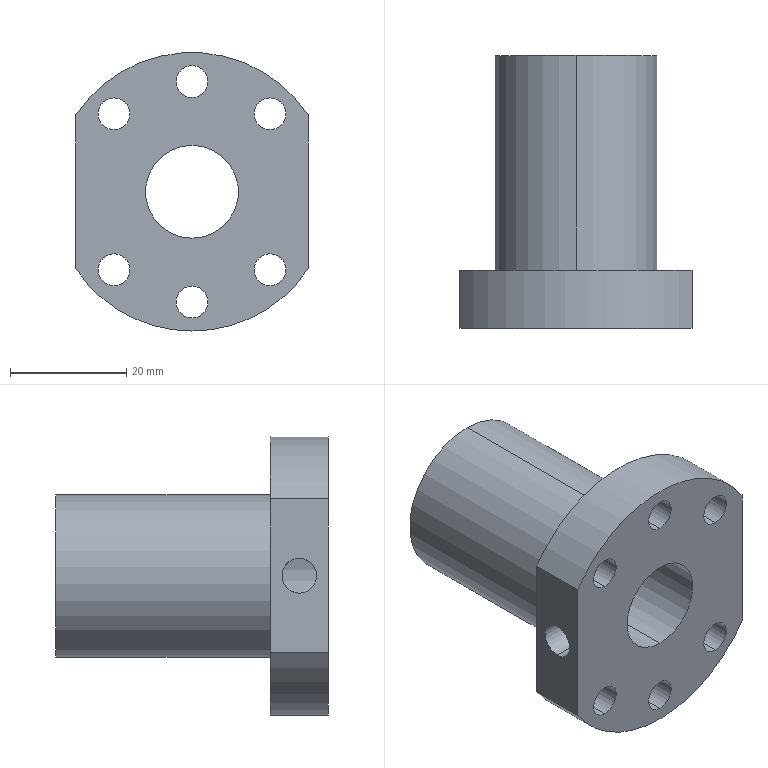Part | SolidWorks | features BaseBody 1 | 1 solid | 26 faces | box 40 x 47 x 48 mm | volume 28219 mm3 | cylinder 21 | plane 5 | commonest cylinder face diameters 5.5 x12 48 x3 6 x2 16 x2 28 x2
STEP:
#1=CARTESIAN_POINT('',(0.,47.,-14.));
#2=VERTEX_POINT('',#1);
#3=CARTESIAN_POINT('',(0.,47.,14.));
#4=VERTEX_POINT('',#3);
#5=CARTESIAN_POINT('',(0.,47.,0.));
#6=DIRECTION('',(0.,-1.,0.));
#7=DIRECTION('',(0.,0.,-1.));
#8=AXIS2_PLACEMENT_3D('',#5,#6,#7);
#9=CIRCLE('',#8,14.);
#10=EDGE_CURVE('',#2,#4,#9,.T.);
#11=ORIENTED_EDGE('',*,*,#10,.T.);
#12=CARTESIAN_POINT('',(0.,10.,14.));
#13=VERTEX_POINT('',#12);
#14=CARTESIAN_POINT('',(0.,47.,14.));
#15=DIRECTION('',(0.,-1.,0.));
#16=VECTOR('',#15,1000.);
#17=LINE('',#14,#16);
#18=EDGE_CURVE('',#4,#13,#17,.T.);
#19=ORIENTED_EDGE('',*,*,#18,.T.);
#20=CARTESIAN_POINT('',(0.,10.,-14.));
#21=VERTEX_POINT('',#20);
#22=CARTESIAN_POINT('',(0.,10.,0.));
#23=DIRECTION('',(0.,1.,0.));
#24=DIRECTION('',(0.,0.,-1.));
#25=AXIS2_PLACEMENT_3D('',#22,#23,#24);
#26=CIRCLE('',#25,14.);
#27=EDGE_CURVE('',#13,#21,#26,.T.);
#28=ORIENTED_EDGE('',*,*,#27,.T.);
#29=CARTESIAN_POINT('',(0.,47.,-14.));
#30=DIRECTION('',(0.,-1.,0.));
#31=VECTOR('',#30,1000.);
#32=LINE('',#29,#31);
#33=EDGE_CURVE('',#2,#21,#32,.T.);
#34=ORIENTED_EDGE('',*,*,#33,.F.);
#35=EDGE_LOOP('',(#11,#19,#28,#34));
#36=FACE_OUTER_BOUND('',#35,.T.);
#37=CARTESIAN_POINT('',(0.,47.,0.));
#38=DIRECTION('',(0.,-1.,0.));
#39=DIRECTION('',(0.,0.,-1.));
#40=AXIS2_PLACEMENT_3D('',#37,#38,#39);
#41=CYLINDRICAL_SURFACE('',#40,14.);
#42=ADVANCED_FACE('',(#36),#41,.T.);
#43=CARTESIAN_POINT('',(-13.435,10.,-10.685));
#44=VERTEX_POINT('',#43);
#45=CARTESIAN_POINT('',(-13.435,10.,-16.185));
#46=VERTEX_POINT('',#45);
#47=CARTESIAN_POINT('',(-13.435,10.,-13.435));
#48=DIRECTION('',(0.,-1.,0.));
#49=DIRECTION('',(0.,0.,-1.));
#50=AXIS2_PLACEMENT_3D('',#47,#48,#49);
#51=CIRCLE('',#50,2.75);
#52=EDGE_CURVE('',#44,#46,#51,.T.);
#53=ORIENTED_EDGE('',*,*,#52,.F.);
#54=CARTESIAN_POINT('',(-13.435,0.,-10.685));
#55=VERTEX_POINT('',#54);
#56=CARTESIAN_POINT('',(-13.435,10.,-10.685));
#57=DIRECTION('',(0.,-1.,0.));
#58=VECTOR('',#57,1000.);
#59=LINE('',#56,#58);
#60=EDGE_CURVE('',#44,#55,#59,.T.);
#61=ORIENTED_EDGE('',*,*,#60,.T.);
#62=CARTESIAN_POINT('',(-13.435,0.,-16.185));
#63=VERTEX_POINT('',#62);
#64=CARTESIAN_POINT('',(-13.435,0.,-13.435));
#65=DIRECTION('',(0.,1.,0.));
#66=DIRECTION('',(0.,0.,-1.));
#67=AXIS2_PLACEMENT_3D('',#64,#65,#66);
#68=CIRCLE('',#67,2.75);
#69=EDGE_CURVE('',#63,#55,#68,.T.);
#70=ORIENTED_EDGE('',*,*,#69,.F.);
#71=CARTESIAN_POINT('',(-13.435,10.,-16.185));
#72=DIRECTION('',(0.,-1.,0.));
#73=VECTOR('',#72,1000.);
#74=LINE('',#71,#73);
#75=EDGE_CURVE('',#46,#63,#74,.T.);
#76=ORIENTED_EDGE('',*,*,#75,.F.);
#77=EDGE_LOOP('',(#53,#61,#70,#76));
#78=FACE_OUTER_BOUND('',#77,.T.);
#79=CARTESIAN_POINT('',(-13.435,10.,-13.435));
#80=DIRECTION('',(0.,-1.,0.));
#81=DIRECTION('',(0.,0.,-1.));
#82=AXIS2_PLACEMENT_3D('',#79,#80,#81);
#83=CYLINDRICAL_SURFACE('',#82,2.75);
#84=ADVANCED_FACE('',(#78),#83,.F.);
#85=CARTESIAN_POINT('',(13.435,10.,16.185));
#86=VERTEX_POINT('',#85);
#87=CARTESIAN_POINT('',(13.435,10.,10.685));
#88=VERTEX_POINT('',#87);
#89=CARTESIAN_POINT('',(13.435,10.,13.435));
#90=DIRECTION('',(0.,-1.,0.));
#91=DIRECTION('',(0.,0.,-1.));
#92=AXIS2_PLACEMENT_3D('',#89,#90,#91);
#93=CIRCLE('',#92,2.75);
#94=EDGE_CURVE('',#86,#88,#93,.T.);
#95=ORIENTED_EDGE('',*,*,#94,.F.);
#96=CARTESIAN_POINT('',(13.435,0.,16.185));
#97=VERTEX_POINT('',#96);
#98=CARTESIAN_POINT('',(13.435,10.,16.185));
#99=DIRECTION('',(0.,-1.,0.));
#100=VECTOR('',#99,1000.);
#101=LINE('',#98,#100);
#102=EDGE_CURVE('',#86,#97,#101,.T.);
#103=ORIENTED_EDGE('',*,*,#102,.T.);
#104=CARTESIAN_POINT('',(13.435,0.,10.685));
#105=VERTEX_POINT('',#104);
#106=CARTESIAN_POINT('',(13.435,0.,13.435));
#107=DIRECTION('',(0.,1.,0.));
#108=DIRECTION('',(0.,0.,-1.));
#109=AXIS2_PLACEMENT_3D('',#106,#107,#108);
#110=CIRCLE('',#109,2.75);
#111=EDGE_CURVE('',#105,#97,#110,.T.);
#112=ORIENTED_EDGE('',*,*,#111,.F.);
#113=CARTESIAN_POINT('',(13.435,10.,10.685));
#114=DIRECTION('',(0.,-1.,0.));
#115=VECTOR('',#114,1000.);
#116=LINE('',#113,#115);
#117=EDGE_CURVE('',#88,#105,#116,.T.);
#118=ORIENTED_EDGE('',*,*,#117,.F.);
#119=EDGE_LOOP('',(#95,#103,#112,#118));
#120=FACE_OUTER_BOUND('',#119,.T.);
#121=CARTESIAN_POINT('',(13.435,10.,13.435));
#122=DIRECTION('',(0.,-1.,0.));
#123=DIRECTION('',(0.,0.,-1.));
#124=AXIS2_PLACEMENT_3D('',#121,#122,#123);
#125=CYLINDRICAL_SURFACE('',#124,2.75);
#126=ADVANCED_FACE('',(#120),#125,.F.);
#127=CARTESIAN_POINT('',(-13.435,10.,16.185));
#128=VERTEX_POINT('',#127);
#129=CARTESIAN_POINT('',(-13.435,10.,10.685));
#130=VERTEX_POINT('',#129);
#131=CARTESIAN_POINT('',(-13.435,10.,13.435));
#132=DIRECTION('',(0.,-1.,0.));
#133=DIRECTION('',(0.,0.,-1.));
#134=AXIS2_PLACEMENT_3D('',#131,#132,#133);
#135=CIRCLE('',#134,2.75);
#136=EDGE_CURVE('',#128,#130,#135,.T.);
#137=ORIENTED_EDGE('',*,*,#136,.F.);
#138=CARTESIAN_POINT('',(-13.435,0.,16.185));
#139=VERTEX_POINT('',#138);
#140=CARTESIAN_POINT('',(-13.435,10.,16.185));
#141=DIRECTION('',(0.,-1.,0.));
#142=VECTOR('',#141,1000.);
#143=LINE('',#140,#142);
#144=EDGE_CURVE('',#128,#139,#143,.T.);
#145=ORIENTED_EDGE('',*,*,#144,.T.);
#146=CARTESIAN_POINT('',(-13.435,0.,10.685));
#147=VERTEX_POINT('',#146);
#148=CARTESIAN_POINT('',(-13.435,0.,13.435));
#149=DIRECTION('',(0.,1.,0.));
#150=DIRECTION('',(0.,0.,-1.));
#151=AXIS2_PLACEMENT_3D('',#148,#149,#150);
#152=CIRCLE('',#151,2.75);
#153=EDGE_CURVE('',#147,#139,#152,.T.);
#154=ORIENTED_EDGE('',*,*,#153,.F.);
#155=CARTESIAN_POINT('',(-13.435,10.,10.685));
#156=DIRECTION('',(0.,-1.,0.));
#157=VECTOR('',#156,1000.);
#158=LINE('',#155,#157);
#159=EDGE_CURVE('',#130,#147,#158,.T.);
#160=ORIENTED_EDGE('',*,*,#159,.F.);
#161=EDGE_LOOP('',(#137,#145,#154,#160));
#162=FACE_OUTER_BOUND('',#161,.T.);
#163=CARTESIAN_POINT('',(-13.435,10.,13.435));
#164=DIRECTION('',(0.,-1.,0.));
#165=DIRECTION('',(0.,0.,-1.));
#166=AXIS2_PLACEMENT_3D('',#163,#164,#165);
#167=CYLINDRICAL_SURFACE('',#166,2.75);
#168=ADVANCED_FACE('',(#162),#167,.F.);
#169=CARTESIAN_POINT('',(0.,10.,21.75));
#170=VERTEX_POINT('',#169);
#171=CARTESIAN_POINT('',(0.,10.,16.25));
#172=VERTEX_POINT('',#171);
#173=CARTESIAN_POINT('',(0.,10.,19.));
#174=DIRECTION('',(0.,-1.,0.));
#175=DIRECTION('',(0.,0.,-1.));
#176=AXIS2_PLACEMENT_3D('',#173,#174,#175);
#177=CIRCLE('',#176,2.75);
#178=EDGE_CURVE('',#170,#172,#177,.T.);
#179=ORIENTED_EDGE('',*,*,#178,.F.);
#180=CARTESIAN_POINT('',(0.,0.,21.75));
#181=VERTEX_POINT('',#180);
#182=CARTESIAN_POINT('',(0.,10.,21.75));
#183=DIRECTION('',(0.,-1.,0.));
#184=VECTOR('',#183,1000.);
#185=LINE('',#182,#184);
#186=EDGE_CURVE('',#170,#181,#185,.T.);
#187=ORIENTED_EDGE('',*,*,#186,.T.);
#188=CARTESIAN_POINT('',(0.,0.,16.25));
#189=VERTEX_POINT('',#188);
#190=CARTESIAN_POINT('',(0.,0.,19.));
#191=DIRECTION('',(0.,1.,0.));
#192=DIRECTION('',(0.,0.,-1.));
#193=AXIS2_PLACEMENT_3D('',#190,#191,#192);
#194=CIRCLE('',#193,2.75);
#195=EDGE_CURVE('',#189,#181,#194,.T.);
#196=ORIENTED_EDGE('',*,*,#195,.F.);
#197=CARTESIAN_POINT('',(0.,10.,16.25));
#198=DIRECTION('',(0.,-1.,0.));
#199=VECTOR('',#198,1000.);
#200=LINE('',#197,#199);
#201=EDGE_CURVE('',#172,#189,#200,.T.);
#202=ORIENTED_EDGE('',*,*,#201,.F.);
#203=EDGE_LOOP('',(#179,#187,#196,#202));
#204=FACE_OUTER_BOUND('',#203,.T.);
#205=CARTESIAN_POINT('',(0.,10.,19.));
#206=DIRECTION('',(0.,-1.,0.));
#207=DIRECTION('',(0.,0.,-1.));
#208=AXIS2_PLACEMENT_3D('',#205,#206,#207);
#209=CYLINDRICAL_SURFACE('',#208,2.75);
#210=ADVANCED_FACE('',(#204),#209,.F.);
#211=CARTESIAN_POINT('',(0.,10.,-24.));
#212=VERTEX_POINT('',#211);
#213=CARTESIAN_POINT('',(-20.,10.,-13.266));
#214=VERTEX_POINT('',#213);
#215=CARTESIAN_POINT('',(0.,10.,0.));
#216=DIRECTION('',(0.,1.,0.));
#217=DIRECTION('',(0.,0.,-1.));
#218=AXIS2_PLACEMENT_3D('',#215,#216,#217);
#219=CIRCLE('',#218,24.);
#220=EDGE_CURVE('',#212,#214,#219,.T.);
#221=ORIENTED_EDGE('',*,*,#220,.F.);
#222=CARTESIAN_POINT('',(0.,0.,-24.));
#223=VERTEX_POINT('',#222);
#224=CARTESIAN_POINT('',(0.,10.,-24.));
#225=DIRECTION('',(0.,-1.,0.));
#226=VECTOR('',#225,1000.);
#227=LINE('',#224,#226);
#228=EDGE_CURVE('',#212,#223,#227,.T.);
#229=ORIENTED_EDGE('',*,*,#228,.T.);
#230=CARTESIAN_POINT('',(-20.,0.,-13.266));
#231=VERTEX_POINT('',#230);
#232=CARTESIAN_POINT('',(0.,0.,0.));
#233=DIRECTION('',(0.,1.,0.));
#234=DIRECTION('',(0.,0.,-1.));
#235=AXIS2_PLACEMENT_3D('',#232,#233,#234);
#236=CIRCLE('',#235,24.);
#237=EDGE_CURVE('',#223,#231,#236,.T.);
#238=ORIENTED_EDGE('',*,*,#237,.T.);
#239=CARTESIAN_POINT('',(-20.,10.,-13.266));
#240=DIRECTION('',(0.,1.,0.));
#241=VECTOR('',#240,1000.);
#242=LINE('',#239,#241);
#243=EDGE_CURVE('',#231,#214,#242,.T.);
#244=ORIENTED_EDGE('',*,*,#243,.T.);
#245=EDGE_LOOP('',(#221,#229,#238,#244));
#246=FACE_OUTER_BOUND('',#245,.T.);
#247=CARTESIAN_POINT('',(0.,10.,0.));
#248=DIRECTION('',(0.,-1.,0.));
#249=DIRECTION('',(0.,0.,-1.));
#250=AXIS2_PLACEMENT_3D('',#247,#248,#249);
#251=CYLINDRICAL_SURFACE('',#250,24.);
#252=ADVANCED_FACE('',(#246),#251,.T.);
#253=CARTESIAN_POINT('',(13.435,10.,-10.685));
#254=VERTEX_POINT('',#253);
#255=CARTESIAN_POINT('',(13.435,10.,-16.185));
#256=VERTEX_POINT('',#255);
#257=CARTESIAN_POINT('',(13.435,10.,-13.435));
#258=DIRECTION('',(0.,-1.,0.));
#259=DIRECTION('',(0.,0.,-1.));
#260=AXIS2_PLACEMENT_3D('',#257,#258,#259);
#261=CIRCLE('',#260,2.75);
#262=EDGE_CURVE('',#254,#256,#261,.T.);
#263=ORIENTED_EDGE('',*,*,#262,.F.);
#264=CARTESIAN_POINT('',(13.435,0.,-10.685));
#265=VERTEX_POINT('',#264);
#266=CARTESIAN_POINT('',(13.435,10.,-10.685));
#267=DIRECTION('',(0.,-1.,0.));
#268=VECTOR('',#267,1000.);
#269=LINE('',#266,#268);
#270=EDGE_CURVE('',#254,#265,#269,.T.);
#271=ORIENTED_EDGE('',*,*,#270,.T.);
#272=CARTESIAN_POINT('',(13.435,0.,-16.185));
#273=VERTEX_POINT('',#272);
#274=CARTESIAN_POINT('',(13.435,0.,-13.435));
#275=DIRECTION('',(0.,1.,0.));
#276=DIRECTION('',(0.,0.,-1.));
#277=AXIS2_PLACEMENT_3D('',#274,#275,#276);
#278=CIRCLE('',#277,2.75);
#279=EDGE_CURVE('',#273,#265,#278,.T.);
#280=ORIENTED_EDGE('',*,*,#279,.F.);
#281=CARTESIAN_POINT('',(13.435,10.,-16.185));
#282=DIRECTION('',(0.,-1.,0.));
#283=VECTOR('',#282,1000.);
#284=LINE('',#281,#283);
#285=EDGE_CURVE('',#256,#273,#284,.T.);
#286=ORIENTED_EDGE('',*,*,#285,.F.);
#287=EDGE_LOOP('',(#263,#271,#280,#286));
#288=FACE_OUTER_BOUND('',#287,.T.);
#289=CARTESIAN_POINT('',(13.435,10.,-13.435));
#290=DIRECTION('',(0.,-1.,0.));
#291=DIRECTION('',(0.,0.,-1.));
#292=AXIS2_PLACEMENT_3D('',#289,#290,#291);
#293=CYLINDRICAL_SURFACE('',#292,2.75);
#294=ADVANCED_FACE('',(#288),#293,.F.);
#295=CARTESIAN_POINT('',(0.,10.,-16.25));
#296=VERTEX_POINT('',#295);
#297=CARTESIAN_POINT('',(0.,10.,-21.75));
#298=VERTEX_POINT('',#297);
#299=CARTESIAN_POINT('',(0.,10.,-19.));
#300=DIRECTION('',(0.,-1.,0.));
#301=DIRECTION('',(0.,0.,-1.));
#302=AXIS2_PLACEMENT_3D('',#299,#300,#301);
#303=CIRCLE('',#302,2.75);
#304=EDGE_CURVE('',#296,#298,#303,.T.);
#305=ORIENTED_EDGE('',*,*,#304,.F.);
#306=CARTESIAN_POINT('',(0.,0.,-16.25));
#307=VERTEX_POINT('',#306);
#308=CARTESIAN_POINT('',(0.,10.,-16.25));
#309=DIRECTION('',(0.,-1.,0.));
#310=VECTOR('',#309,1000.);
#311=LINE('',#308,#310);
#312=EDGE_CURVE('',#296,#307,#311,.T.);
#313=ORIENTED_EDGE('',*,*,#312,.T.);
#314=CARTESIAN_POINT('',(0.,0.,-21.75));
#315=VERTEX_POINT('',#314);
#316=CARTESIAN_POINT('',(0.,0.,-19.));
#317=DIRECTION('',(0.,1.,0.));
#318=DIRECTION('',(0.,0.,-1.));
#319=AXIS2_PLACEMENT_3D('',#316,#317,#318);
#320=CIRCLE('',#319,2.75);
#321=EDGE_CURVE('',#315,#307,#320,.T.);
#322=ORIENTED_EDGE('',*,*,#321,.F.);
#323=CARTESIAN_POINT('',(0.,10.,-21.75));
#324=DIRECTION('',(0.,-1.,0.));
#325=VECTOR('',#324,1000.);
#326=LINE('',#323,#325);
#327=EDGE_CURVE('',#298,#315,#326,.T.);
#328=ORIENTED_EDGE('',*,*,#327,.F.);
#329=EDGE_LOOP('',(#305,#313,#322,#328));
#330=FACE_OUTER_BOUND('',#329,.T.);
#331=CARTESIAN_POINT('',(0.,10.,-19.));
#332=DIRECTION('',(0.,-1.,0.));
#333=DIRECTION('',(0.,0.,-1.));
#334=AXIS2_PLACEMENT_3D('',#331,#332,#333);
#335=CYLINDRICAL_SURFACE('',#334,2.75);
#336=ADVANCED_FACE('',(#330),#335,.F.);
#337=CARTESIAN_POINT('',(-7.416,5.,3.));
#338=VERTEX_POINT('',#337);
#339=CARTESIAN_POINT('',(-7.416,5.,-3.));
#340=VERTEX_POINT('',#339);
#341=CARTESIAN_POINT('',(-7.416,5.,3.));
#342=CARTESIAN_POINT('',(-7.416,4.8,3.));
#343=CARTESIAN_POINT('',(-7.424,4.603,2.98));
#344=CARTESIAN_POINT('',(-7.455,4.218,2.903));
#345=CARTESIAN_POINT('',(-7.478,4.026,2.844));
#346=CARTESIAN_POINT('',(-7.533,3.664,2.693));
#347=CARTESIAN_POINT('',(-7.566,3.493,2.601));
#348=CARTESIAN_POINT('',(-7.637,3.168,2.384));
#349=CARTESIAN_POINT('',(-7.676,3.016,2.259));
#350=CARTESIAN_POINT('',(-7.789,2.605,1.848));
#351=CARTESIAN_POINT('',(-7.863,2.382,1.516));
#352=CARTESIAN_POINT('',(-7.942,2.157,0.9761));
#353=CARTESIAN_POINT('',(-7.964,2.098,0.7852));
#354=CARTESIAN_POINT('',(-7.993,2.02,0.3971));
#355=CARTESIAN_POINT('',(-8.,2.,0.2012));
#356=CARTESIAN_POINT('',(-8.,2.,-0.1942));
#357=CARTESIAN_POINT('',(-7.993,2.02,-0.3949));
#358=CARTESIAN_POINT('',(-7.964,2.097,-0.7814));
#359=CARTESIAN_POINT('',(-7.943,2.154,-0.9694));
#360=CARTESIAN_POINT('',(-7.89,2.306,-1.335));
#361=CARTESIAN_POINT('',(-7.858,2.399,-1.507));
#362=CARTESIAN_POINT('',(-7.789,2.615,-1.831));
#363=CARTESIAN_POINT('',(-7.752,2.741,-1.983));
#364=CARTESIAN_POINT('',(-7.676,3.016,-2.259));
#365=CARTESIAN_POINT('',(-7.638,3.165,-2.382));
#366=CARTESIAN_POINT('',(-7.567,3.489,-2.599));
#367=CARTESIAN_POINT('',(-7.534,3.664,-2.693));
#368=CARTESIAN_POINT('',(-7.478,4.024,-2.844));
#369=CARTESIAN_POINT('',(-7.456,4.211,-2.901));
#370=CARTESIAN_POINT('',(-7.424,4.6,-2.98));
#371=CARTESIAN_POINT('',(-7.416,4.8,-3.));
#372=CARTESIAN_POINT('',(-7.416,5.,-3.));
#373=B_SPLINE_CURVE_WITH_KNOTS('',3,(#341,#342,#343,#344,#345,#346,#347,#348,#349,#350,#351,#352,#353,#354,#355,#356,#357,#358,#359,#360,#361,#362,#363,#364,#365,#366,#367,#368,#369,#370,#371,#372),.UNSPECIFIED.,.F.,.F.,(4,2,2,2,2,2,2,2,2,2,2,2,2,2,2,4),(0.,0.0005914,0.001183,0.001774,0.002366,0.003548,0.00414,0.004731,0.005323,0.005914,0.006505,0.007097,0.007688,0.00828,0.008871,0.009462),.UNSPECIFIED.);
#374=EDGE_CURVE('',#338,#340,#373,.T.);
#375=ORIENTED_EDGE('',*,*,#374,.F.);
#376=CARTESIAN_POINT('',(-7.416,5.,-3.));
#377=CARTESIAN_POINT('',(-7.416,5.2,-3.));
#378=CARTESIAN_POINT('',(-7.424,5.397,-2.98));
#379=CARTESIAN_POINT('',(-7.455,5.782,-2.903));
#380=CARTESIAN_POINT('',(-7.478,5.974,-2.844));
#381=CARTESIAN_POINT('',(-7.533,6.336,-2.693));
#382=CARTESIAN_POINT('',(-7.566,6.507,-2.601));
#383=CARTESIAN_POINT('',(-7.637,6.832,-2.384));
#384=CARTESIAN_POINT('',(-7.676,6.984,-2.259));
#385=CARTESIAN_POINT('',(-7.789,7.395,-1.848));
#386=CARTESIAN_POINT('',(-7.863,7.618,-1.516));
#387=CARTESIAN_POINT('',(-7.942,7.843,-0.9761));
#388=CARTESIAN_POINT('',(-7.964,7.902,-0.7852));
#389=CARTESIAN_POINT('',(-7.993,7.98,-0.3971));
#390=CARTESIAN_POINT('',(-8.,8.,-0.2012));
#391=CARTESIAN_POINT('',(-8.,8.,0.1942));
#392=CARTESIAN_POINT('',(-7.993,7.98,0.3949));
#393=CARTESIAN_POINT('',(-7.964,7.903,0.7814));
#394=CARTESIAN_POINT('',(-7.943,7.846,0.9694));
#395=CARTESIAN_POINT('',(-7.89,7.694,1.335));
#396=CARTESIAN_POINT('',(-7.858,7.601,1.507));
#397=CARTESIAN_POINT('',(-7.789,7.385,1.831));
#398=CARTESIAN_POINT('',(-7.752,7.259,1.983));
#399=CARTESIAN_POINT('',(-7.676,6.984,2.259));
#400=CARTESIAN_POINT('',(-7.638,6.835,2.382));
#401=CARTESIAN_POINT('',(-7.567,6.511,2.599));
#402=CARTESIAN_POINT('',(-7.534,6.336,2.693));
#403=CARTESIAN_POINT('',(-7.478,5.976,2.844));
#404=CARTESIAN_POINT('',(-7.456,5.789,2.901));
#405=CARTESIAN_POINT('',(-7.424,5.4,2.98));
#406=CARTESIAN_POINT('',(-7.416,5.2,3.));
#407=CARTESIAN_POINT('',(-7.416,5.,3.));
#408=B_SPLINE_CURVE_WITH_KNOTS('',3,(#376,#377,#378,#379,#380,#381,#382,#383,#384,#385,#386,#387,#388,#389,#390,#391,#392,#393,#394,#395,#396,#397,#398,#399,#400,#401,#402,#403,#404,#405,#406,#407),.UNSPECIFIED.,.F.,.F.,(4,2,2,2,2,2,2,2,2,2,2,2,2,2,2,4),(0.009462,0.01005,0.01064,0.01124,0.01183,0.01301,0.0136,0.01419,0.01478,0.01538,0.01597,0.01656,0.01715,0.01774,0.01833,0.01892),.UNSPECIFIED.);
#409=EDGE_CURVE('',#340,#338,#408,.T.);
#410=ORIENTED_EDGE('',*,*,#409,.F.);
#411=EDGE_LOOP('',(#375,#410));
#412=FACE_BOUND('',#411,.T.);
#413=CARTESIAN_POINT('',(0.,47.,8.));
#414=VERTEX_POINT('',#413);
#415=CARTESIAN_POINT('',(0.,47.,-8.));
#416=VERTEX_POINT('',#415);
#417=CARTESIAN_POINT('',(0.,47.,0.));
#418=DIRECTION('',(0.,-1.,0.));
#419=DIRECTION('',(0.,0.,-1.));
#420=AXIS2_PLACEMENT_3D('',#417,#418,#419);
#421=CIRCLE('',#420,8.);
#422=EDGE_CURVE('',#414,#416,#421,.T.);
#423=ORIENTED_EDGE('',*,*,#422,.F.);
#424=CARTESIAN_POINT('',(0.,0.,8.));
#425=VERTEX_POINT('',#424);
#426=CARTESIAN_POINT('',(0.,47.,8.));
#427=DIRECTION('',(0.,-1.,0.));
#428=VECTOR('',#427,1000.);
#429=LINE('',#426,#428);
#430=EDGE_CURVE('',#414,#425,#429,.T.);
#431=ORIENTED_EDGE('',*,*,#430,.T.);
#432=CARTESIAN_POINT('',(0.,0.,-8.));
#433=VERTEX_POINT('',#432);
#434=CARTESIAN_POINT('',(0.,0.,0.));
#435=DIRECTION('',(0.,1.,0.));
#436=DIRECTION('',(0.,0.,-1.));
#437=AXIS2_PLACEMENT_3D('',#434,#435,#436);
#438=CIRCLE('',#437,8.);
#439=EDGE_CURVE('',#433,#425,#438,.T.);
#440=ORIENTED_EDGE('',*,*,#439,.F.);
#441=CARTESIAN_POINT('',(0.,47.,-8.));
#442=DIRECTION('',(0.,-1.,0.));
#443=VECTOR('',#442,1000.);
#444=LINE('',#441,#443);
#445=EDGE_CURVE('',#416,#433,#444,.T.);
#446=ORIENTED_EDGE('',*,*,#445,.F.);
#447=EDGE_LOOP('',(#423,#431,#440,#446));
#448=FACE_OUTER_BOUND('',#447,.T.);
#449=CARTESIAN_POINT('',(0.,47.,0.));
#450=DIRECTION('',(0.,-1.,0.));
#451=DIRECTION('',(0.,0.,-1.));
#452=AXIS2_PLACEMENT_3D('',#449,#450,#451);
#453=CYLINDRICAL_SURFACE('',#452,8.);
#454=ADVANCED_FACE('',(#412,#448),#453,.F.);
#455=ORIENTED_EDGE('',*,*,#374,.T.);
#456=CARTESIAN_POINT('',(-20.,5.,-3.));
#457=VERTEX_POINT('',#456);
#458=CARTESIAN_POINT('',(0.,5.,-3.));
#459=DIRECTION('',(-1.,0.,0.));
#460=VECTOR('',#459,1000.);
#461=LINE('',#458,#460);
#462=EDGE_CURVE('',#340,#457,#461,.T.);
#463=ORIENTED_EDGE('',*,*,#462,.T.);
#464=CARTESIAN_POINT('',(-20.,5.,3.));
#465=VERTEX_POINT('',#464);
#466=CARTESIAN_POINT('',(-20.,5.,0.));
#467=DIRECTION('',(-1.,0.,0.));
#468=DIRECTION('',(0.,0.,1.));
#469=AXIS2_PLACEMENT_3D('',#466,#467,#468);
#470=CIRCLE('',#469,3.);
#471=EDGE_CURVE('',#457,#465,#470,.T.);
#472=ORIENTED_EDGE('',*,*,#471,.T.);
#473=CARTESIAN_POINT('',(0.,5.,3.));
#474=DIRECTION('',(-1.,0.,0.));
#475=VECTOR('',#474,1000.);
#476=LINE('',#473,#475);
#477=EDGE_CURVE('',#338,#465,#476,.T.);
#478=ORIENTED_EDGE('',*,*,#477,.F.);
#479=EDGE_LOOP('',(#455,#463,#472,#478));
#480=FACE_OUTER_BOUND('',#479,.T.);
#481=CARTESIAN_POINT('',(0.,5.,0.));
#482=DIRECTION('',(-1.,0.,0.));
#483=DIRECTION('',(0.,0.,1.));
#484=AXIS2_PLACEMENT_3D('',#481,#482,#483);
#485=CYLINDRICAL_SURFACE('',#484,3.);
#486=ADVANCED_FACE('',(#480),#485,.F.);
#487=ORIENTED_EDGE('',*,*,#18,.F.);
#488=CARTESIAN_POINT('',(0.,47.,0.));
#489=DIRECTION('',(0.,-1.,0.));
#490=DIRECTION('',(0.,0.,-1.));
#491=AXIS2_PLACEMENT_3D('',#488,#489,#490);
#492=CIRCLE('',#491,14.);
#493=EDGE_CURVE('',#4,#2,#492,.T.);
#494=ORIENTED_EDGE('',*,*,#493,.T.);
#495=ORIENTED_EDGE('',*,*,#33,.T.);
#496=CARTESIAN_POINT('',(0.,10.,0.));
#497=DIRECTION('',(0.,1.,0.));
#498=DIRECTION('',(0.,0.,-1.));
#499=AXIS2_PLACEMENT_3D('',#496,#497,#498);
#500=CIRCLE('',#499,14.);
#501=EDGE_CURVE('',#21,#13,#500,.T.);
#502=ORIENTED_EDGE('',*,*,#501,.T.);
#503=EDGE_LOOP('',(#487,#494,#495,#502));
#504=FACE_OUTER_BOUND('',#503,.T.);
#505=CARTESIAN_POINT('',(0.,47.,0.));
#506=DIRECTION('',(0.,-1.,0.));
#507=DIRECTION('',(0.,0.,-1.));
#508=AXIS2_PLACEMENT_3D('',#505,#506,#507);
#509=CYLINDRICAL_SURFACE('',#508,14.);
#510=ADVANCED_FACE('',(#504),#509,.T.);
#511=CARTESIAN_POINT('',(-13.435,10.,-13.435));
#512=DIRECTION('',(0.,-1.,0.));
#513=DIRECTION('',(0.,0.,-1.));
#514=AXIS2_PLACEMENT_3D('',#511,#512,#513);
#515=CIRCLE('',#514,2.75);
#516=EDGE_CURVE('',#46,#44,#515,.T.);
#517=ORIENTED_EDGE('',*,*,#516,.T.);
#518=ORIENTED_EDGE('',*,*,#52,.T.);
#519=EDGE_LOOP('',(#517,#518));
#520=FACE_BOUND('',#519,.T.);
#521=CARTESIAN_POINT('',(13.435,10.,13.435));
#522=DIRECTION('',(0.,-1.,0.));
#523=DIRECTION('',(0.,0.,-1.));
#524=AXIS2_PLACEMENT_3D('',#521,#522,#523);
#525=CIRCLE('',#524,2.75);
#526=EDGE_CURVE('',#88,#86,#525,.T.);
#527=ORIENTED_EDGE('',*,*,#526,.T.);
#528=ORIENTED_EDGE('',*,*,#94,.T.);
#529=EDGE_LOOP('',(#527,#528));
#530=FACE_BOUND('',#529,.T.);
#531=CARTESIAN_POINT('',(-13.435,10.,13.435));
#532=DIRECTION('',(0.,-1.,0.));
#533=DIRECTION('',(0.,0.,-1.));
#534=AXIS2_PLACEMENT_3D('',#531,#532,#533);
#535=CIRCLE('',#534,2.75);
#536=EDGE_CURVE('',#130,#128,#535,.T.);
#537=ORIENTED_EDGE('',*,*,#536,.T.);
#538=ORIENTED_EDGE('',*,*,#136,.T.);
#539=EDGE_LOOP('',(#537,#538));
#540=FACE_BOUND('',#539,.T.);
#541=CARTESIAN_POINT('',(0.,10.,19.));
#542=DIRECTION('',(0.,-1.,0.));
#543=DIRECTION('',(0.,0.,-1.));
#544=AXIS2_PLACEMENT_3D('',#541,#542,#543);
#545=CIRCLE('',#544,2.75);
#546=EDGE_CURVE('',#172,#170,#545,.T.);
#547=ORIENTED_EDGE('',*,*,#546,.T.);
#548=ORIENTED_EDGE('',*,*,#178,.T.);
#549=EDGE_LOOP('',(#547,#548));
#550=FACE_BOUND('',#549,.T.);
#551=ORIENTED_EDGE('',*,*,#501,.F.);
#552=ORIENTED_EDGE('',*,*,#27,.F.);
#553=EDGE_LOOP('',(#551,#552));
#554=FACE_BOUND('',#553,.T.);
#555=CARTESIAN_POINT('',(-20.,10.,13.266));
#556=VERTEX_POINT('',#555);
#557=CARTESIAN_POINT('',(-20.,10.,0.));
#558=DIRECTION('',(0.,0.,1.));
#559=VECTOR('',#558,1000.);
#560=LINE('',#557,#559);
#561=EDGE_CURVE('',#214,#556,#560,.T.);
#562=ORIENTED_EDGE('',*,*,#561,.T.);
#563=CARTESIAN_POINT('',(20.,10.,13.266));
#564=VERTEX_POINT('',#563);
#565=CARTESIAN_POINT('',(0.,10.,0.));
#566=DIRECTION('',(0.,1.,0.));
#567=DIRECTION('',(0.,0.,-1.));
#568=AXIS2_PLACEMENT_3D('',#565,#566,#567);
#569=CIRCLE('',#568,24.);
#570=EDGE_CURVE('',#556,#564,#569,.T.);
#571=ORIENTED_EDGE('',*,*,#570,.T.);
#572=CARTESIAN_POINT('',(20.,10.,-13.266));
#573=VERTEX_POINT('',#572);
#574=CARTESIAN_POINT('',(20.,10.,0.));
#575=DIRECTION('',(0.,0.,-1.));
#576=VECTOR('',#575,1000.);
#577=LINE('',#574,#576);
#578=EDGE_CURVE('',#564,#573,#577,.T.);
#579=ORIENTED_EDGE('',*,*,#578,.T.);
#580=CARTESIAN_POINT('',(0.,10.,0.));
#581=DIRECTION('',(0.,1.,0.));
#582=DIRECTION('',(0.,0.,-1.));
#583=AXIS2_PLACEMENT_3D('',#580,#581,#582);
#584=CIRCLE('',#583,24.);
#585=EDGE_CURVE('',#573,#212,#584,.T.);
#586=ORIENTED_EDGE('',*,*,#585,.T.);
#587=ORIENTED_EDGE('',*,*,#220,.T.);
#588=EDGE_LOOP('',(#562,#571,#579,#586,#587));
#589=FACE_OUTER_BOUND('',#588,.T.);
#590=CARTESIAN_POINT('',(13.435,10.,-13.435));
#591=DIRECTION('',(0.,-1.,0.));
#592=DIRECTION('',(0.,0.,-1.));
#593=AXIS2_PLACEMENT_3D('',#590,#591,#592);
#594=CIRCLE('',#593,2.75);
#595=EDGE_CURVE('',#256,#254,#594,.T.);
#596=ORIENTED_EDGE('',*,*,#595,.T.);
#597=ORIENTED_EDGE('',*,*,#262,.T.);
#598=EDGE_LOOP('',(#596,#597));
#599=FACE_BOUND('',#598,.T.);
#600=CARTESIAN_POINT('',(0.,10.,-19.));
#601=DIRECTION('',(0.,-1.,0.));
#602=DIRECTION('',(0.,0.,-1.));
#603=AXIS2_PLACEMENT_3D('',#600,#601,#602);
#604=CIRCLE('',#603,2.75);
#605=EDGE_CURVE('',#298,#296,#604,.T.);
#606=ORIENTED_EDGE('',*,*,#605,.T.);
#607=ORIENTED_EDGE('',*,*,#304,.T.);
#608=EDGE_LOOP('',(#606,#607));
#609=FACE_BOUND('',#608,.T.);
#610=CARTESIAN_POINT('',(0.,10.,0.));
#611=DIRECTION('',(0.,1.,0.));
#612=DIRECTION('',(0.,0.,1.));
#613=AXIS2_PLACEMENT_3D('',#610,#611,#612);
#614=PLANE('',#613);
#615=ADVANCED_FACE('',(#520,#530,#540,#550,#554,#589,#599,#609),#614,.T.);
#616=ORIENTED_EDGE('',*,*,#10,.F.);
#617=ORIENTED_EDGE('',*,*,#493,.F.);
#618=EDGE_LOOP('',(#616,#617));
#619=FACE_OUTER_BOUND('',#618,.T.);
#620=CARTESIAN_POINT('',(0.,47.,0.));
#621=DIRECTION('',(0.,-1.,0.));
#622=DIRECTION('',(0.,0.,-1.));
#623=AXIS2_PLACEMENT_3D('',#620,#621,#622);
#624=CIRCLE('',#623,8.);
#625=EDGE_CURVE('',#416,#414,#624,.T.);
#626=ORIENTED_EDGE('',*,*,#625,.T.);
#627=ORIENTED_EDGE('',*,*,#422,.T.);
#628=EDGE_LOOP('',(#626,#627));
#629=FACE_BOUND('',#628,.T.);
#630=CARTESIAN_POINT('',(0.,47.,0.));
#631=DIRECTION('',(0.,1.,0.));
#632=DIRECTION('',(0.,0.,1.));
#633=AXIS2_PLACEMENT_3D('',#630,#631,#632);
#634=PLANE('',#633);
#635=ADVANCED_FACE('',(#619,#629),#634,.T.);
#636=ORIENTED_EDGE('',*,*,#60,.F.);
#637=ORIENTED_EDGE('',*,*,#516,.F.);
#638=ORIENTED_EDGE('',*,*,#75,.T.);
#639=CARTESIAN_POINT('',(-13.435,0.,-13.435));
#640=DIRECTION('',(0.,1.,0.));
#641=DIRECTION('',(0.,0.,-1.));
#642=AXIS2_PLACEMENT_3D('',#639,#640,#641);
#643=CIRCLE('',#642,2.75);
#644=EDGE_CURVE('',#55,#63,#643,.T.);
#645=ORIENTED_EDGE('',*,*,#644,.F.);
#646=EDGE_LOOP('',(#636,#637,#638,#645));
#647=FACE_OUTER_BOUND('',#646,.T.);
#648=CARTESIAN_POINT('',(-13.435,10.,-13.435));
#649=DIRECTION('',(0.,-1.,0.));
#650=DIRECTION('',(0.,0.,-1.));
#651=AXIS2_PLACEMENT_3D('',#648,#649,#650);
#652=CYLINDRICAL_SURFACE('',#651,2.75);
#653=ADVANCED_FACE('',(#647),#652,.F.);
#654=ORIENTED_EDGE('',*,*,#102,.F.);
#655=ORIENTED_EDGE('',*,*,#526,.F.);
#656=ORIENTED_EDGE('',*,*,#117,.T.);
#657=CARTESIAN_POINT('',(13.435,0.,13.435));
#658=DIRECTION('',(0.,1.,0.));
#659=DIRECTION('',(0.,0.,-1.));
#660=AXIS2_PLACEMENT_3D('',#657,#658,#659);
#661=CIRCLE('',#660,2.75);
#662=EDGE_CURVE('',#97,#105,#661,.T.);
#663=ORIENTED_EDGE('',*,*,#662,.F.);
#664=EDGE_LOOP('',(#654,#655,#656,#663));
#665=FACE_OUTER_BOUND('',#664,.T.);
#666=CARTESIAN_POINT('',(13.435,10.,13.435));
#667=DIRECTION('',(0.,-1.,0.));
#668=DIRECTION('',(0.,0.,-1.));
#669=AXIS2_PLACEMENT_3D('',#666,#667,#668);
#670=CYLINDRICAL_SURFACE('',#669,2.75);
#671=ADVANCED_FACE('',(#665),#670,.F.);
#672=ORIENTED_EDGE('',*,*,#144,.F.);
#673=ORIENTED_EDGE('',*,*,#536,.F.);
#674=ORIENTED_EDGE('',*,*,#159,.T.);
#675=CARTESIAN_POINT('',(-13.435,0.,13.435));
#676=DIRECTION('',(0.,1.,0.));
#677=DIRECTION('',(0.,0.,-1.));
#678=AXIS2_PLACEMENT_3D('',#675,#676,#677);
#679=CIRCLE('',#678,2.75);
#680=EDGE_CURVE('',#139,#147,#679,.T.);
#681=ORIENTED_EDGE('',*,*,#680,.F.);
#682=EDGE_LOOP('',(#672,#673,#674,#681));
#683=FACE_OUTER_BOUND('',#682,.T.);
#684=CARTESIAN_POINT('',(-13.435,10.,13.435));
#685=DIRECTION('',(0.,-1.,0.));
#686=DIRECTION('',(0.,0.,-1.));
#687=AXIS2_PLACEMENT_3D('',#684,#685,#686);
#688=CYLINDRICAL_SURFACE('',#687,2.75);
#689=ADVANCED_FACE('',(#683),#688,.F.);
#690=ORIENTED_EDGE('',*,*,#186,.F.);
#691=ORIENTED_EDGE('',*,*,#546,.F.);
#692=ORIENTED_EDGE('',*,*,#201,.T.);
#693=CARTESIAN_POINT('',(0.,0.,19.));
#694=DIRECTION('',(0.,1.,0.));
#695=DIRECTION('',(0.,0.,-1.));
#696=AXIS2_PLACEMENT_3D('',#693,#694,#695);
#697=CIRCLE('',#696,2.75);
#698=EDGE_CURVE('',#181,#189,#697,.T.);
#699=ORIENTED_EDGE('',*,*,#698,.F.);
#700=EDGE_LOOP('',(#690,#691,#692,#699));
#701=FACE_OUTER_BOUND('',#700,.T.);
#702=CARTESIAN_POINT('',(0.,10.,19.));
#703=DIRECTION('',(0.,-1.,0.));
#704=DIRECTION('',(0.,0.,-1.));
#705=AXIS2_PLACEMENT_3D('',#702,#703,#704);
#706=CYLINDRICAL_SURFACE('',#705,2.75);
#707=ADVANCED_FACE('',(#701),#706,.F.);
#708=ORIENTED_EDGE('',*,*,#570,.F.);
#709=CARTESIAN_POINT('',(-20.,0.,13.266));
#710=VERTEX_POINT('',#709);
#711=CARTESIAN_POINT('',(-20.,10.,13.266));
#712=DIRECTION('',(0.,-1.,0.));
#713=VECTOR('',#712,1000.);
#714=LINE('',#711,#713);
#715=EDGE_CURVE('',#556,#710,#714,.T.);
#716=ORIENTED_EDGE('',*,*,#715,.T.);
#717=CARTESIAN_POINT('',(20.,0.,13.266));
#718=VERTEX_POINT('',#717);
#719=CARTESIAN_POINT('',(0.,0.,0.));
#720=DIRECTION('',(0.,1.,0.));
#721=DIRECTION('',(0.,0.,-1.));
#722=AXIS2_PLACEMENT_3D('',#719,#720,#721);
#723=CIRCLE('',#722,24.);
#724=EDGE_CURVE('',#710,#718,#723,.T.);
#725=ORIENTED_EDGE('',*,*,#724,.T.);
#726=CARTESIAN_POINT('',(20.,10.,13.266));
#727=DIRECTION('',(0.,1.,0.));
#728=VECTOR('',#727,1000.);
#729=LINE('',#726,#728);
#730=EDGE_CURVE('',#718,#564,#729,.T.);
#731=ORIENTED_EDGE('',*,*,#730,.T.);
#732=EDGE_LOOP('',(#708,#716,#725,#731));
#733=FACE_OUTER_BOUND('',#732,.T.);
#734=CARTESIAN_POINT('',(0.,10.,0.));
#735=DIRECTION('',(0.,-1.,0.));
#736=DIRECTION('',(0.,0.,-1.));
#737=AXIS2_PLACEMENT_3D('',#734,#735,#736);
#738=CYLINDRICAL_SURFACE('',#737,24.);
#739=ADVANCED_FACE('',(#733),#738,.T.);
#740=ORIENTED_EDGE('',*,*,#715,.F.);
#741=ORIENTED_EDGE('',*,*,#561,.F.);
#742=ORIENTED_EDGE('',*,*,#243,.F.);
#743=CARTESIAN_POINT('',(-20.,0.,0.));
#744=DIRECTION('',(0.,0.,-1.));
#745=VECTOR('',#744,1000.);
#746=LINE('',#743,#745);
#747=EDGE_CURVE('',#710,#231,#746,.T.);
#748=ORIENTED_EDGE('',*,*,#747,.F.);
#749=EDGE_LOOP('',(#740,#741,#742,#748));
#750=FACE_OUTER_BOUND('',#749,.T.);
#751=CARTESIAN_POINT('',(-20.,5.,0.));
#752=DIRECTION('',(-1.,0.,0.));
#753=DIRECTION('',(0.,0.,1.));
#754=AXIS2_PLACEMENT_3D('',#751,#752,#753);
#755=CIRCLE('',#754,3.);
#756=EDGE_CURVE('',#465,#457,#755,.T.);
#757=ORIENTED_EDGE('',*,*,#756,.F.);
#758=ORIENTED_EDGE('',*,*,#471,.F.);
#759=EDGE_LOOP('',(#757,#758));
#760=FACE_BOUND('',#759,.T.);
#761=CARTESIAN_POINT('',(-20.,10.,0.));
#762=DIRECTION('',(1.,0.,0.));
#763=DIRECTION('',(0.,0.,-1.));
#764=AXIS2_PLACEMENT_3D('',#761,#762,#763);
#765=PLANE('',#764);
#766=ADVANCED_FACE('',(#750,#760),#765,.F.);
#767=ORIENTED_EDGE('',*,*,#228,.F.);
#768=ORIENTED_EDGE('',*,*,#585,.F.);
#769=CARTESIAN_POINT('',(20.,0.,-13.266));
#770=VERTEX_POINT('',#769);
#771=CARTESIAN_POINT('',(20.,10.,-13.266));
#772=DIRECTION('',(0.,-1.,0.));
#773=VECTOR('',#772,1000.);
#774=LINE('',#771,#773);
#775=EDGE_CURVE('',#573,#770,#774,.T.);
#776=ORIENTED_EDGE('',*,*,#775,.T.);
#777=CARTESIAN_POINT('',(0.,0.,0.));
#778=DIRECTION('',(0.,1.,0.));
#779=DIRECTION('',(0.,0.,-1.));
#780=AXIS2_PLACEMENT_3D('',#777,#778,#779);
#781=CIRCLE('',#780,24.);
#782=EDGE_CURVE('',#770,#223,#781,.T.);
#783=ORIENTED_EDGE('',*,*,#782,.T.);
#784=EDGE_LOOP('',(#767,#768,#776,#783));
#785=FACE_OUTER_BOUND('',#784,.T.);
#786=CARTESIAN_POINT('',(0.,10.,0.));
#787=DIRECTION('',(0.,-1.,0.));
#788=DIRECTION('',(0.,0.,-1.));
#789=AXIS2_PLACEMENT_3D('',#786,#787,#788);
#790=CYLINDRICAL_SURFACE('',#789,24.);
#791=ADVANCED_FACE('',(#785),#790,.T.);
#792=ORIENTED_EDGE('',*,*,#578,.F.);
#793=ORIENTED_EDGE('',*,*,#730,.F.);
#794=CARTESIAN_POINT('',(20.,0.,0.));
#795=DIRECTION('',(0.,0.,-1.));
#796=VECTOR('',#795,1000.);
#797=LINE('',#794,#796);
#798=EDGE_CURVE('',#718,#770,#797,.T.);
#799=ORIENTED_EDGE('',*,*,#798,.T.);
#800=ORIENTED_EDGE('',*,*,#775,.F.);
#801=EDGE_LOOP('',(#792,#793,#799,#800));
#802=FACE_OUTER_BOUND('',#801,.T.);
#803=CARTESIAN_POINT('',(20.,10.,0.));
#804=DIRECTION('',(1.,0.,0.));
#805=DIRECTION('',(0.,0.,-1.));
#806=AXIS2_PLACEMENT_3D('',#803,#804,#805);
#807=PLANE('',#806);
#808=ADVANCED_FACE('',(#802),#807,.T.);
#809=ORIENTED_EDGE('',*,*,#270,.F.);
#810=ORIENTED_EDGE('',*,*,#595,.F.);
#811=ORIENTED_EDGE('',*,*,#285,.T.);
#812=CARTESIAN_POINT('',(13.435,0.,-13.435));
#813=DIRECTION('',(0.,1.,0.));
#814=DIRECTION('',(0.,0.,-1.));
#815=AXIS2_PLACEMENT_3D('',#812,#813,#814);
#816=CIRCLE('',#815,2.75);
#817=EDGE_CURVE('',#265,#273,#816,.T.);
#818=ORIENTED_EDGE('',*,*,#817,.F.);
#819=EDGE_LOOP('',(#809,#810,#811,#818));
#820=FACE_OUTER_BOUND('',#819,.T.);
#821=CARTESIAN_POINT('',(13.435,10.,-13.435));
#822=DIRECTION('',(0.,-1.,0.));
#823=DIRECTION('',(0.,0.,-1.));
#824=AXIS2_PLACEMENT_3D('',#821,#822,#823);
#825=CYLINDRICAL_SURFACE('',#824,2.75);
#826=ADVANCED_FACE('',(#820),#825,.F.);
#827=ORIENTED_EDGE('',*,*,#312,.F.);
#828=ORIENTED_EDGE('',*,*,#605,.F.);
#829=ORIENTED_EDGE('',*,*,#327,.T.);
#830=CARTESIAN_POINT('',(0.,0.,-19.));
#831=DIRECTION('',(0.,1.,0.));
#832=DIRECTION('',(0.,0.,-1.));
#833=AXIS2_PLACEMENT_3D('',#830,#831,#832);
#834=CIRCLE('',#833,2.75);
#835=EDGE_CURVE('',#307,#315,#834,.T.);
#836=ORIENTED_EDGE('',*,*,#835,.F.);
#837=EDGE_LOOP('',(#827,#828,#829,#836));
#838=FACE_OUTER_BOUND('',#837,.T.);
#839=CARTESIAN_POINT('',(0.,10.,-19.));
#840=DIRECTION('',(0.,-1.,0.));
#841=DIRECTION('',(0.,0.,-1.));
#842=AXIS2_PLACEMENT_3D('',#839,#840,#841);
#843=CYLINDRICAL_SURFACE('',#842,2.75);
#844=ADVANCED_FACE('',(#838),#843,.F.);
#845=ORIENTED_EDGE('',*,*,#430,.F.);
#846=ORIENTED_EDGE('',*,*,#625,.F.);
#847=ORIENTED_EDGE('',*,*,#445,.T.);
#848=CARTESIAN_POINT('',(0.,0.,0.));
#849=DIRECTION('',(0.,1.,0.));
#850=DIRECTION('',(0.,0.,-1.));
#851=AXIS2_PLACEMENT_3D('',#848,#849,#850);
#852=CIRCLE('',#851,8.);
#853=EDGE_CURVE('',#425,#433,#852,.T.);
#854=ORIENTED_EDGE('',*,*,#853,.F.);
#855=EDGE_LOOP('',(#845,#846,#847,#854));
#856=FACE_OUTER_BOUND('',#855,.T.);
#857=CARTESIAN_POINT('',(0.,47.,0.));
#858=DIRECTION('',(0.,-1.,0.));
#859=DIRECTION('',(0.,0.,-1.));
#860=AXIS2_PLACEMENT_3D('',#857,#858,#859);
#861=CYLINDRICAL_SURFACE('',#860,8.);
#862=ADVANCED_FACE('',(#856),#861,.F.);
#863=ORIENTED_EDGE('',*,*,#439,.T.);
#864=ORIENTED_EDGE('',*,*,#853,.T.);
#865=EDGE_LOOP('',(#863,#864));
#866=FACE_BOUND('',#865,.T.);
#867=ORIENTED_EDGE('',*,*,#69,.T.);
#868=ORIENTED_EDGE('',*,*,#644,.T.);
#869=EDGE_LOOP('',(#867,#868));
#870=FACE_BOUND('',#869,.T.);
#871=ORIENTED_EDGE('',*,*,#111,.T.);
#872=ORIENTED_EDGE('',*,*,#662,.T.);
#873=EDGE_LOOP('',(#871,#872));
#874=FACE_BOUND('',#873,.T.);
#875=ORIENTED_EDGE('',*,*,#153,.T.);
#876=ORIENTED_EDGE('',*,*,#680,.T.);
#877=EDGE_LOOP('',(#875,#876));
#878=FACE_BOUND('',#877,.T.);
#879=ORIENTED_EDGE('',*,*,#195,.T.);
#880=ORIENTED_EDGE('',*,*,#698,.T.);
#881=EDGE_LOOP('',(#879,#880));
#882=FACE_BOUND('',#881,.T.);
#883=ORIENTED_EDGE('',*,*,#724,.F.);
#884=ORIENTED_EDGE('',*,*,#747,.T.);
#885=ORIENTED_EDGE('',*,*,#237,.F.);
#886=ORIENTED_EDGE('',*,*,#782,.F.);
#887=ORIENTED_EDGE('',*,*,#798,.F.);
#888=EDGE_LOOP('',(#883,#884,#885,#886,#887));
#889=FACE_OUTER_BOUND('',#888,.T.);
#890=ORIENTED_EDGE('',*,*,#279,.T.);
#891=ORIENTED_EDGE('',*,*,#817,.T.);
#892=EDGE_LOOP('',(#890,#891));
#893=FACE_BOUND('',#892,.T.);
#894=ORIENTED_EDGE('',*,*,#321,.T.);
#895=ORIENTED_EDGE('',*,*,#835,.T.);
#896=EDGE_LOOP('',(#894,#895));
#897=FACE_BOUND('',#896,.T.);
#898=CARTESIAN_POINT('',(0.,0.,0.));
#899=DIRECTION('',(0.,1.,0.));
#900=DIRECTION('',(0.,0.,1.));
#901=AXIS2_PLACEMENT_3D('',#898,#899,#900);
#902=PLANE('',#901);
#903=ADVANCED_FACE('',(#866,#870,#874,#878,#882,#889,#893,#897),#902,.F.);
#904=ORIENTED_EDGE('',*,*,#462,.F.);
#905=ORIENTED_EDGE('',*,*,#409,.T.);
#906=ORIENTED_EDGE('',*,*,#477,.T.);
#907=ORIENTED_EDGE('',*,*,#756,.T.);
#908=EDGE_LOOP('',(#904,#905,#906,#907));
#909=FACE_OUTER_BOUND('',#908,.T.);
#910=CARTESIAN_POINT('',(0.,5.,0.));
#911=DIRECTION('',(-1.,0.,0.));
#912=DIRECTION('',(0.,0.,1.));
#913=AXIS2_PLACEMENT_3D('',#910,#911,#912);
#914=CYLINDRICAL_SURFACE('',#913,3.);
#915=ADVANCED_FACE('',(#909),#914,.F.);
#916=CLOSED_SHELL('',(#42,#84,#126,#168,#210,#252,#294,#336,#454,#486,#510,#615,#635,#653,#671,#689,#707,#739,#766,#791,#808,#826,#844,#862,#903,#915));
#917=MANIFOLD_SOLID_BREP('',#916);
#918=CARTESIAN_POINT('',(0.,0.,0.));
#919=DIRECTION('',(0.,0.,1.));
#920=DIRECTION('',(1.,0.,0.));
#921=AXIS2_PLACEMENT_3D('',#918,#919,#920);
#922=(LENGTH_UNIT()NAMED_UNIT(*)SI_UNIT(.MILLI.,.METRE.));
#923=UNCERTAINTY_MEASURE_WITH_UNIT(LENGTH_MEASURE(0.00001),#922,'','');
#924=(NAMED_UNIT(*)PLANE_ANGLE_UNIT()SI_UNIT($,.RADIAN.));
#925=(NAMED_UNIT(*)SI_UNIT($,.STERADIAN.)SOLID_ANGLE_UNIT());
#926=(GEOMETRIC_REPRESENTATION_CONTEXT(3)GLOBAL_UNCERTAINTY_ASSIGNED_CONTEXT((#923))GLOBAL_UNIT_ASSIGNED_CONTEXT((#922,#924,#925))REPRESENTATION_CONTEXT('',''));
#927=ADVANCED_BREP_SHAPE_REPRESENTATION('',(#917,#921),#926);